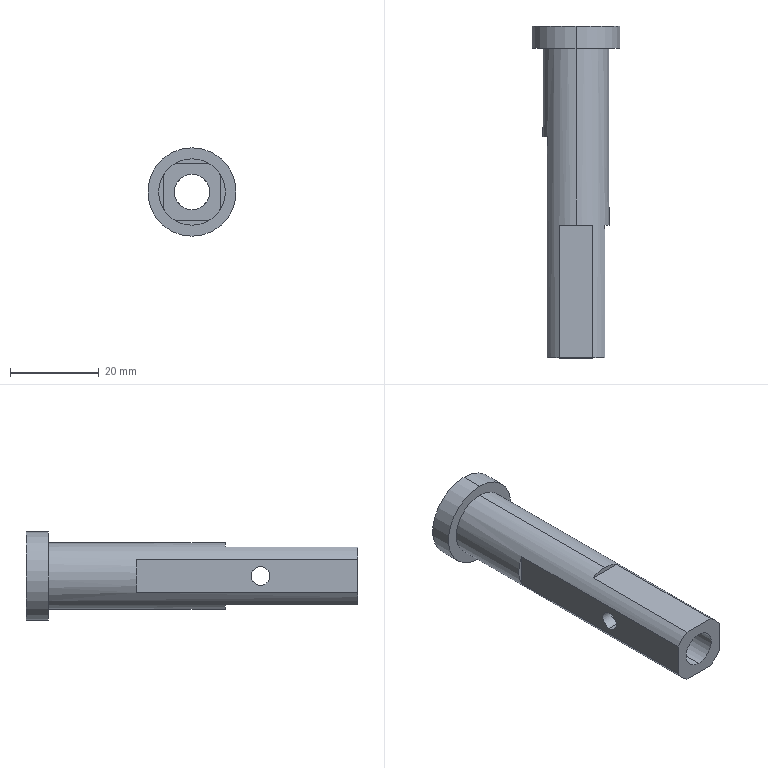Part | SolidWorks | features BaseBody 1 | 1 solid | 21 faces | box 20 x 75 x 20 mm | volume 9389 mm3 | plane 11 | cylinder 10 | commonest cylinder face diameters 4.2 x4 8 x2 15 x2 20 x2
STEP:
#1=CARTESIAN_POINT('',(-6.5,22.,2.1));
#2=VERTEX_POINT('',#1);
#3=CARTESIAN_POINT('',(-3.404,22.,2.1));
#4=VERTEX_POINT('',#3);
#5=CARTESIAN_POINT('',(6.5,22.,2.1));
#6=DIRECTION('',(1.,0.,0.));
#7=VECTOR('',#6,1000.);
#8=LINE('',#5,#7);
#9=EDGE_CURVE('',#2,#4,#8,.T.);
#10=ORIENTED_EDGE('',*,*,#9,.F.);
#11=CARTESIAN_POINT('',(-6.5,22.,-2.1));
#12=VERTEX_POINT('',#11);
#13=CARTESIAN_POINT('',(-6.5,22.,0.));
#14=DIRECTION('',(1.,0.,0.));
#15=DIRECTION('',(0.,0.,-1.));
#16=AXIS2_PLACEMENT_3D('',#13,#14,#15);
#17=CIRCLE('',#16,2.1);
#18=EDGE_CURVE('',#12,#2,#17,.T.);
#19=ORIENTED_EDGE('',*,*,#18,.F.);
#20=CARTESIAN_POINT('',(-3.404,22.,-2.1));
#21=VERTEX_POINT('',#20);
#22=CARTESIAN_POINT('',(6.5,22.,-2.1));
#23=DIRECTION('',(1.,0.,0.));
#24=VECTOR('',#23,1000.);
#25=LINE('',#22,#24);
#26=EDGE_CURVE('',#12,#21,#25,.T.);
#27=ORIENTED_EDGE('',*,*,#26,.T.);
#28=CARTESIAN_POINT('',(-3.404,22.,2.1));
#29=CARTESIAN_POINT('',(-3.404,22.139,2.1));
#30=CARTESIAN_POINT('',(-3.413,22.277,2.087));
#31=CARTESIAN_POINT('',(-3.437,22.48,2.046));
#32=CARTESIAN_POINT('',(-3.447,22.547,2.029));
#33=CARTESIAN_POINT('',(-3.465,22.647,1.998));
#34=CARTESIAN_POINT('',(-3.472,22.681,1.987));
#35=CARTESIAN_POINT('',(-3.485,22.747,1.963));
#36=CARTESIAN_POINT('',(-3.493,22.782,1.949));
#37=CARTESIAN_POINT('',(-3.529,22.938,1.884));
#38=CARTESIAN_POINT('',(-3.563,23.056,1.821));
#39=CARTESIAN_POINT('',(-3.617,23.224,1.708));
#40=CARTESIAN_POINT('',(-3.636,23.278,1.668));
#41=CARTESIAN_POINT('',(-3.675,23.384,1.581));
#42=CARTESIAN_POINT('',(-3.695,23.436,1.534));
#43=CARTESIAN_POINT('',(-3.753,23.582,1.388));
#44=CARTESIAN_POINT('',(-3.79,23.668,1.284));
#45=CARTESIAN_POINT('',(-3.842,23.781,1.116));
#46=CARTESIAN_POINT('',(-3.858,23.816,1.058));
#47=CARTESIAN_POINT('',(-3.889,23.88,0.9387));
#48=CARTESIAN_POINT('',(-3.903,23.909,0.8786));
#49=CARTESIAN_POINT('',(-3.97,24.045,0.5543));
#50=CARTESIAN_POINT('',(-4.,24.1,0.2829));
#51=CARTESIAN_POINT('',(-4.,24.1,-0.138));
#52=CARTESIAN_POINT('',(-3.993,24.087,-0.2764));
#53=CARTESIAN_POINT('',(-3.972,24.046,-0.4803));
#54=CARTESIAN_POINT('',(-3.963,24.029,-0.5476));
#55=CARTESIAN_POINT('',(-3.942,23.988,-0.6808));
#56=CARTESIAN_POINT('',(-3.93,23.963,-0.7482));
#57=CARTESIAN_POINT('',(-3.89,23.883,-0.9392));
#58=CARTESIAN_POINT('',(-3.859,23.819,-1.059));
#59=CARTESIAN_POINT('',(-3.79,23.668,-1.284));
#60=CARTESIAN_POINT('',(-3.753,23.582,-1.388));
#61=CARTESIAN_POINT('',(-3.674,23.385,-1.585));
#62=CARTESIAN_POINT('',(-3.635,23.279,-1.671));
#63=CARTESIAN_POINT('',(-3.581,23.112,-1.783));
#64=CARTESIAN_POINT('',(-3.563,23.054,-1.818));
#65=CARTESIAN_POINT('',(-3.538,22.966,-1.865));
#66=CARTESIAN_POINT('',(-3.53,22.936,-1.881));
#67=CARTESIAN_POINT('',(-3.515,22.875,-1.909));
#68=CARTESIAN_POINT('',(-3.508,22.846,-1.922));
#69=CARTESIAN_POINT('',(-3.439,22.55,-2.047));
#70=CARTESIAN_POINT('',(-3.404,22.279,-2.1));
#71=CARTESIAN_POINT('',(-3.404,22.,-2.1));
#72=B_SPLINE_CURVE_WITH_KNOTS('',3,(#28,#29,#30,#31,#32,#33,#34,#35,#36,#37,#38,#39,#40,#41,#42,#43,#44,#45,#46,#47,#48,#49,#50,#51,#52,#53,#54,#55,#56,#57,#58,#59,#60,#61,#62,#63,#64,#65,#66,#67,#68,#69,#70,#71),.UNSPECIFIED.,.F.,.F.,(4,2,2,2,2,2,2,2,2,2,2,2,2,2,2,2,2,2,2,2,2,4),(0.,0.0625,0.09375,0.1094,0.125,0.1875,0.2188,0.25,0.3125,0.3438,0.375,0.5,0.5625,0.5938,0.625,0.6875,0.75,0.8125,0.8438,0.8594,0.875,1.),.UNSPECIFIED.);
#73=EDGE_CURVE('',#4,#21,#72,.T.);
#74=ORIENTED_EDGE('',*,*,#73,.F.);
#75=EDGE_LOOP('',(#10,#19,#27,#74));
#76=FACE_OUTER_BOUND('',#75,.T.);
#77=CARTESIAN_POINT('',(6.5,22.,0.));
#78=DIRECTION('',(1.,0.,0.));
#79=DIRECTION('',(0.,0.,-1.));
#80=AXIS2_PLACEMENT_3D('',#77,#78,#79);
#81=CYLINDRICAL_SURFACE('',#80,2.1);
#82=ADVANCED_FACE('',(#76),#81,.F.);
#83=CARTESIAN_POINT('',(3.404,22.,2.1));
#84=VERTEX_POINT('',#83);
#85=CARTESIAN_POINT('',(6.5,22.,2.1));
#86=VERTEX_POINT('',#85);
#87=CARTESIAN_POINT('',(6.5,22.,2.1));
#88=DIRECTION('',(1.,0.,0.));
#89=VECTOR('',#88,1000.);
#90=LINE('',#87,#89);
#91=EDGE_CURVE('',#84,#86,#90,.T.);
#92=ORIENTED_EDGE('',*,*,#91,.F.);
#93=CARTESIAN_POINT('',(3.404,22.,-2.1));
#94=VERTEX_POINT('',#93);
#95=CARTESIAN_POINT('',(3.404,22.,-2.1));
#96=CARTESIAN_POINT('',(3.404,22.139,-2.1));
#97=CARTESIAN_POINT('',(3.413,22.277,-2.087));
#98=CARTESIAN_POINT('',(3.437,22.48,-2.046));
#99=CARTESIAN_POINT('',(3.447,22.547,-2.029));
#100=CARTESIAN_POINT('',(3.465,22.647,-1.998));
#101=CARTESIAN_POINT('',(3.472,22.681,-1.987));
#102=CARTESIAN_POINT('',(3.485,22.747,-1.963));
#103=CARTESIAN_POINT('',(3.493,22.782,-1.949));
#104=CARTESIAN_POINT('',(3.515,22.875,-1.91));
#105=CARTESIAN_POINT('',(3.53,22.936,-1.881));
#106=CARTESIAN_POINT('',(3.564,23.056,-1.817));
#107=CARTESIAN_POINT('',(3.582,23.116,-1.78));
#108=CARTESIAN_POINT('',(3.637,23.284,-1.667));
#109=CARTESIAN_POINT('',(3.675,23.388,-1.582));
#110=CARTESIAN_POINT('',(3.752,23.58,-1.39));
#111=CARTESIAN_POINT('',(3.79,23.666,-1.286));
#112=CARTESIAN_POINT('',(3.842,23.78,-1.116));
#113=CARTESIAN_POINT('',(3.858,23.815,-1.058));
#114=CARTESIAN_POINT('',(3.881,23.864,-0.968));
#115=CARTESIAN_POINT('',(3.889,23.879,-0.9378));
#116=CARTESIAN_POINT('',(3.903,23.909,-0.8765));
#117=CARTESIAN_POINT('',(3.91,23.922,-0.8465));
#118=CARTESIAN_POINT('',(3.97,24.045,-0.5542));
#119=CARTESIAN_POINT('',(4.,24.1,-0.2827));
#120=CARTESIAN_POINT('',(4.,24.1,0.1391));
#121=CARTESIAN_POINT('',(3.993,24.086,0.2779));
#122=CARTESIAN_POINT('',(3.971,24.045,0.4822));
#123=CARTESIAN_POINT('',(3.958,24.02,0.5833));
#124=CARTESIAN_POINT('',(3.941,23.986,0.6829));
#125=CARTESIAN_POINT('',(3.929,23.962,0.7489));
#126=CARTESIAN_POINT('',(3.923,23.949,0.7827));
#127=CARTESIAN_POINT('',(3.864,23.83,1.067));
#128=CARTESIAN_POINT('',(3.79,23.675,1.296));
#129=CARTESIAN_POINT('',(3.694,23.434,1.536));
#130=CARTESIAN_POINT('',(3.675,23.384,1.581));
#131=CARTESIAN_POINT('',(3.637,23.28,1.666));
#132=CARTESIAN_POINT('',(3.618,23.227,1.706));
#133=CARTESIAN_POINT('',(3.581,23.112,1.783));
#134=CARTESIAN_POINT('',(3.563,23.053,1.818));
#135=CARTESIAN_POINT('',(3.538,22.964,1.866));
#136=CARTESIAN_POINT('',(3.53,22.934,1.881));
#137=CARTESIAN_POINT('',(3.514,22.873,1.91));
#138=CARTESIAN_POINT('',(3.507,22.844,1.923));
#139=CARTESIAN_POINT('',(3.439,22.548,2.047));
#140=CARTESIAN_POINT('',(3.404,22.278,2.1));
#141=CARTESIAN_POINT('',(3.404,22.,2.1));
#142=B_SPLINE_CURVE_WITH_KNOTS('',3,(#95,#96,#97,#98,#99,#100,#101,#102,#103,#104,#105,#106,#107,#108,#109,#110,#111,#112,#113,#114,#115,#116,#117,#118,#119,#120,#121,#122,#123,#124,#125,#126,#127,#128,#129,#130,#131,#132,#133,#134,#135,#136,#137,#138,#139,#140,#141),.UNSPECIFIED.,.F.,.F.,(4,2,2,2,2,2,2,2,2,2,2,2,2,2,1,2,2,2,2,2,2,2,2,4),(0.,0.0625,0.09375,0.1094,0.125,0.1562,0.1875,0.25,0.3125,0.3437,0.3594,0.375,0.5,0.5625,0.5937,0.6094,0.625,0.75,0.7813,0.8125,0.8438,0.8594,0.875,1.),.UNSPECIFIED.);
#143=EDGE_CURVE('',#94,#84,#142,.T.);
#144=ORIENTED_EDGE('',*,*,#143,.F.);
#145=CARTESIAN_POINT('',(6.5,22.,-2.1));
#146=VERTEX_POINT('',#145);
#147=CARTESIAN_POINT('',(6.5,22.,-2.1));
#148=DIRECTION('',(1.,0.,0.));
#149=VECTOR('',#148,1000.);
#150=LINE('',#147,#149);
#151=EDGE_CURVE('',#94,#146,#150,.T.);
#152=ORIENTED_EDGE('',*,*,#151,.T.);
#153=CARTESIAN_POINT('',(6.5,22.,0.));
#154=DIRECTION('',(1.,0.,0.));
#155=DIRECTION('',(0.,0.,-1.));
#156=AXIS2_PLACEMENT_3D('',#153,#154,#155);
#157=CIRCLE('',#156,2.1);
#158=EDGE_CURVE('',#146,#86,#157,.T.);
#159=ORIENTED_EDGE('',*,*,#158,.T.);
#160=EDGE_LOOP('',(#92,#144,#152,#159));
#161=FACE_OUTER_BOUND('',#160,.T.);
#162=CARTESIAN_POINT('',(6.5,22.,0.));
#163=DIRECTION('',(1.,0.,0.));
#164=DIRECTION('',(0.,0.,-1.));
#165=AXIS2_PLACEMENT_3D('',#162,#163,#164);
#166=CYLINDRICAL_SURFACE('',#165,2.1);
#167=ADVANCED_FACE('',(#161),#166,.F.);
#168=CARTESIAN_POINT('',(-3.742,30.,6.5));
#169=VERTEX_POINT('',#168);
#170=CARTESIAN_POINT('',(3.742,30.,6.5));
#171=VERTEX_POINT('',#170);
#172=CARTESIAN_POINT('',(-5.,30.,6.5));
#173=DIRECTION('',(1.,0.,0.));
#174=VECTOR('',#173,1000.);
#175=LINE('',#172,#174);
#176=EDGE_CURVE('',#169,#171,#175,.T.);
#177=ORIENTED_EDGE('',*,*,#176,.T.);
#178=CARTESIAN_POINT('',(0.,30.,7.5));
#179=VERTEX_POINT('',#178);
#180=CARTESIAN_POINT('',(0.,30.,0.));
#181=DIRECTION('',(0.,1.,0.));
#182=DIRECTION('',(0.,0.,1.));
#183=AXIS2_PLACEMENT_3D('',#180,#181,#182);
#184=CIRCLE('',#183,7.5);
#185=EDGE_CURVE('',#179,#171,#184,.T.);
#186=ORIENTED_EDGE('',*,*,#185,.F.);
#187=CARTESIAN_POINT('',(0.,30.,0.));
#188=DIRECTION('',(0.,1.,0.));
#189=DIRECTION('',(0.,0.,1.));
#190=AXIS2_PLACEMENT_3D('',#187,#188,#189);
#191=CIRCLE('',#190,7.5);
#192=EDGE_CURVE('',#169,#179,#191,.T.);
#193=ORIENTED_EDGE('',*,*,#192,.F.);
#194=EDGE_LOOP('',(#177,#186,#193));
#195=FACE_OUTER_BOUND('',#194,.T.);
#196=CARTESIAN_POINT('',(0.,30.,0.));
#197=DIRECTION('',(0.,1.,0.));
#198=DIRECTION('',(1.,0.,0.));
#199=AXIS2_PLACEMENT_3D('',#196,#197,#198);
#200=PLANE('',#199);
#201=ADVANCED_FACE('',(#195),#200,.F.);
#202=ORIENTED_EDGE('',*,*,#176,.F.);
#203=CARTESIAN_POINT('',(-3.742,0.,6.5));
#204=VERTEX_POINT('',#203);
#205=CARTESIAN_POINT('',(-3.742,0.,6.5));
#206=DIRECTION('',(0.,1.,0.));
#207=VECTOR('',#206,1000.);
#208=LINE('',#205,#207);
#209=EDGE_CURVE('',#204,#169,#208,.T.);
#210=ORIENTED_EDGE('',*,*,#209,.F.);
#211=CARTESIAN_POINT('',(3.742,0.,6.5));
#212=VERTEX_POINT('',#211);
#213=CARTESIAN_POINT('',(-5.,0.,6.5));
#214=DIRECTION('',(1.,0.,0.));
#215=VECTOR('',#214,1000.);
#216=LINE('',#213,#215);
#217=EDGE_CURVE('',#204,#212,#216,.T.);
#218=ORIENTED_EDGE('',*,*,#217,.T.);
#219=CARTESIAN_POINT('',(3.742,0.,6.5));
#220=DIRECTION('',(0.,-1.,0.));
#221=VECTOR('',#220,1000.);
#222=LINE('',#219,#221);
#223=EDGE_CURVE('',#171,#212,#222,.T.);
#224=ORIENTED_EDGE('',*,*,#223,.F.);
#225=EDGE_LOOP('',(#202,#210,#218,#224));
#226=FACE_OUTER_BOUND('',#225,.T.);
#227=CARTESIAN_POINT('',(-5.,30.,6.5));
#228=DIRECTION('',(0.,0.,-1.));
#229=DIRECTION('',(0.,-1.,0.));
#230=AXIS2_PLACEMENT_3D('',#227,#228,#229);
#231=PLANE('',#230);
#232=ADVANCED_FACE('',(#226),#231,.F.);
#233=CARTESIAN_POINT('',(-3.742,30.,-6.5));
#234=VERTEX_POINT('',#233);
#235=CARTESIAN_POINT('',(0.,30.,-7.5));
#236=VERTEX_POINT('',#235);
#237=CARTESIAN_POINT('',(0.,30.,0.));
#238=DIRECTION('',(0.,-1.,0.));
#239=DIRECTION('',(0.,0.,-1.));
#240=AXIS2_PLACEMENT_3D('',#237,#238,#239);
#241=CIRCLE('',#240,7.5);
#242=EDGE_CURVE('',#234,#236,#241,.T.);
#243=ORIENTED_EDGE('',*,*,#242,.T.);
#244=CARTESIAN_POINT('',(3.742,30.,-6.5));
#245=VERTEX_POINT('',#244);
#246=CARTESIAN_POINT('',(0.,30.,0.));
#247=DIRECTION('',(0.,-1.,0.));
#248=DIRECTION('',(0.,0.,-1.));
#249=AXIS2_PLACEMENT_3D('',#246,#247,#248);
#250=CIRCLE('',#249,7.5);
#251=EDGE_CURVE('',#236,#245,#250,.T.);
#252=ORIENTED_EDGE('',*,*,#251,.T.);
#253=CARTESIAN_POINT('',(-5.,30.,-6.5));
#254=DIRECTION('',(-1.,0.,0.));
#255=VECTOR('',#254,1000.);
#256=LINE('',#253,#255);
#257=EDGE_CURVE('',#245,#234,#256,.T.);
#258=ORIENTED_EDGE('',*,*,#257,.T.);
#259=EDGE_LOOP('',(#243,#252,#258));
#260=FACE_OUTER_BOUND('',#259,.T.);
#261=CARTESIAN_POINT('',(0.,30.,0.));
#262=DIRECTION('',(0.,-1.,0.));
#263=DIRECTION('',(0.,0.,-1.));
#264=AXIS2_PLACEMENT_3D('',#261,#262,#263);
#265=PLANE('',#264);
#266=ADVANCED_FACE('',(#260),#265,.T.);
#267=ORIENTED_EDGE('',*,*,#257,.F.);
#268=CARTESIAN_POINT('',(3.742,0.,-6.5));
#269=VERTEX_POINT('',#268);
#270=CARTESIAN_POINT('',(3.742,0.,-6.5));
#271=DIRECTION('',(0.,1.,0.));
#272=VECTOR('',#271,1000.);
#273=LINE('',#270,#272);
#274=EDGE_CURVE('',#269,#245,#273,.T.);
#275=ORIENTED_EDGE('',*,*,#274,.F.);
#276=CARTESIAN_POINT('',(-3.742,0.,-6.5));
#277=VERTEX_POINT('',#276);
#278=CARTESIAN_POINT('',(-5.,0.,-6.5));
#279=DIRECTION('',(-1.,0.,0.));
#280=VECTOR('',#279,1000.);
#281=LINE('',#278,#280);
#282=EDGE_CURVE('',#269,#277,#281,.T.);
#283=ORIENTED_EDGE('',*,*,#282,.T.);
#284=CARTESIAN_POINT('',(-3.742,0.,-6.5));
#285=DIRECTION('',(0.,-1.,0.));
#286=VECTOR('',#285,1000.);
#287=LINE('',#284,#286);
#288=EDGE_CURVE('',#234,#277,#287,.T.);
#289=ORIENTED_EDGE('',*,*,#288,.F.);
#290=EDGE_LOOP('',(#267,#275,#283,#289));
#291=FACE_OUTER_BOUND('',#290,.T.);
#292=CARTESIAN_POINT('',(-5.,30.,-6.5));
#293=DIRECTION('',(0.,0.,1.));
#294=DIRECTION('',(1.,0.,0.));
#295=AXIS2_PLACEMENT_3D('',#292,#293,#294);
#296=PLANE('',#295);
#297=ADVANCED_FACE('',(#291),#296,.F.);
#298=CARTESIAN_POINT('',(6.5,30.,3.742));
#299=VERTEX_POINT('',#298);
#300=CARTESIAN_POINT('',(6.5,30.,-3.742));
#301=VERTEX_POINT('',#300);
#302=CARTESIAN_POINT('',(6.5,30.,-5.));
#303=DIRECTION('',(0.,0.,-1.));
#304=VECTOR('',#303,1000.);
#305=LINE('',#302,#304);
#306=EDGE_CURVE('',#299,#301,#305,.T.);
#307=ORIENTED_EDGE('',*,*,#306,.T.);
#308=CARTESIAN_POINT('',(0.,30.,0.));
#309=DIRECTION('',(0.,1.,0.));
#310=DIRECTION('',(0.,0.,1.));
#311=AXIS2_PLACEMENT_3D('',#308,#309,#310);
#312=CIRCLE('',#311,7.5);
#313=EDGE_CURVE('',#299,#301,#312,.T.);
#314=ORIENTED_EDGE('',*,*,#313,.F.);
#315=EDGE_LOOP('',(#307,#314));
#316=FACE_OUTER_BOUND('',#315,.T.);
#317=CARTESIAN_POINT('',(0.,30.,0.));
#318=DIRECTION('',(0.,1.,0.));
#319=DIRECTION('',(1.,0.,0.));
#320=AXIS2_PLACEMENT_3D('',#317,#318,#319);
#321=PLANE('',#320);
#322=ADVANCED_FACE('',(#316),#321,.F.);
#323=ORIENTED_EDGE('',*,*,#158,.F.);
#324=CARTESIAN_POINT('',(6.5,22.,0.));
#325=DIRECTION('',(1.,0.,0.));
#326=DIRECTION('',(0.,0.,-1.));
#327=AXIS2_PLACEMENT_3D('',#324,#325,#326);
#328=CIRCLE('',#327,2.1);
#329=EDGE_CURVE('',#86,#146,#328,.T.);
#330=ORIENTED_EDGE('',*,*,#329,.F.);
#331=EDGE_LOOP('',(#323,#330));
#332=FACE_BOUND('',#331,.T.);
#333=ORIENTED_EDGE('',*,*,#306,.F.);
#334=CARTESIAN_POINT('',(6.5,0.,3.742));
#335=VERTEX_POINT('',#334);
#336=CARTESIAN_POINT('',(6.5,0.,3.742));
#337=DIRECTION('',(0.,1.,0.));
#338=VECTOR('',#337,1000.);
#339=LINE('',#336,#338);
#340=EDGE_CURVE('',#335,#299,#339,.T.);
#341=ORIENTED_EDGE('',*,*,#340,.F.);
#342=CARTESIAN_POINT('',(6.5,0.,-3.742));
#343=VERTEX_POINT('',#342);
#344=CARTESIAN_POINT('',(6.5,0.,-5.));
#345=DIRECTION('',(0.,0.,-1.));
#346=VECTOR('',#345,1000.);
#347=LINE('',#344,#346);
#348=EDGE_CURVE('',#335,#343,#347,.T.);
#349=ORIENTED_EDGE('',*,*,#348,.T.);
#350=CARTESIAN_POINT('',(6.5,0.,-3.742));
#351=DIRECTION('',(0.,-1.,0.));
#352=VECTOR('',#351,1000.);
#353=LINE('',#350,#352);
#354=EDGE_CURVE('',#301,#343,#353,.T.);
#355=ORIENTED_EDGE('',*,*,#354,.F.);
#356=EDGE_LOOP('',(#333,#341,#349,#355));
#357=FACE_OUTER_BOUND('',#356,.T.);
#358=CARTESIAN_POINT('',(6.5,30.,-5.));
#359=DIRECTION('',(-1.,0.,0.));
#360=DIRECTION('',(0.,0.,1.));
#361=AXIS2_PLACEMENT_3D('',#358,#359,#360);
#362=PLANE('',#361);
#363=ADVANCED_FACE('',(#332,#357),#362,.F.);
#364=CARTESIAN_POINT('',(-6.5,50.,3.742));
#365=VERTEX_POINT('',#364);
#366=CARTESIAN_POINT('',(-6.5,50.,-3.742));
#367=VERTEX_POINT('',#366);
#368=CARTESIAN_POINT('',(0.,50.,0.));
#369=DIRECTION('',(0.,-1.,0.));
#370=DIRECTION('',(0.,0.,-1.));
#371=AXIS2_PLACEMENT_3D('',#368,#369,#370);
#372=CIRCLE('',#371,7.5);
#373=EDGE_CURVE('',#365,#367,#372,.T.);
#374=ORIENTED_EDGE('',*,*,#373,.T.);
#375=CARTESIAN_POINT('',(-6.5,50.,0.));
#376=DIRECTION('',(0.,0.,1.));
#377=VECTOR('',#376,1000.);
#378=LINE('',#375,#377);
#379=EDGE_CURVE('',#367,#365,#378,.T.);
#380=ORIENTED_EDGE('',*,*,#379,.T.);
#381=EDGE_LOOP('',(#374,#380));
#382=FACE_OUTER_BOUND('',#381,.T.);
#383=CARTESIAN_POINT('',(0.,50.,0.));
#384=DIRECTION('',(0.,-1.,0.));
#385=DIRECTION('',(0.,0.,-1.));
#386=AXIS2_PLACEMENT_3D('',#383,#384,#385);
#387=PLANE('',#386);
#388=ADVANCED_FACE('',(#382),#387,.T.);
#389=ORIENTED_EDGE('',*,*,#18,.T.);
#390=CARTESIAN_POINT('',(-6.5,22.,0.));
#391=DIRECTION('',(1.,0.,0.));
#392=DIRECTION('',(0.,0.,-1.));
#393=AXIS2_PLACEMENT_3D('',#390,#391,#392);
#394=CIRCLE('',#393,2.1);
#395=EDGE_CURVE('',#2,#12,#394,.T.);
#396=ORIENTED_EDGE('',*,*,#395,.T.);
#397=EDGE_LOOP('',(#389,#396));
#398=FACE_BOUND('',#397,.T.);
#399=ORIENTED_EDGE('',*,*,#379,.F.);
#400=CARTESIAN_POINT('',(-6.5,0.,-3.742));
#401=VERTEX_POINT('',#400);
#402=CARTESIAN_POINT('',(-6.5,0.,-3.742));
#403=DIRECTION('',(0.,1.,0.));
#404=VECTOR('',#403,1000.);
#405=LINE('',#402,#404);
#406=EDGE_CURVE('',#401,#367,#405,.T.);
#407=ORIENTED_EDGE('',*,*,#406,.F.);
#408=CARTESIAN_POINT('',(-6.5,0.,3.742));
#409=VERTEX_POINT('',#408);
#410=CARTESIAN_POINT('',(-6.5,0.,-5.));
#411=DIRECTION('',(0.,0.,1.));
#412=VECTOR('',#411,1000.);
#413=LINE('',#410,#412);
#414=EDGE_CURVE('',#401,#409,#413,.T.);
#415=ORIENTED_EDGE('',*,*,#414,.T.);
#416=CARTESIAN_POINT('',(-6.5,0.,3.742));
#417=DIRECTION('',(0.,-1.,0.));
#418=VECTOR('',#417,1000.);
#419=LINE('',#416,#418);
#420=EDGE_CURVE('',#365,#409,#419,.T.);
#421=ORIENTED_EDGE('',*,*,#420,.F.);
#422=EDGE_LOOP('',(#399,#407,#415,#421));
#423=FACE_OUTER_BOUND('',#422,.T.);
#424=CARTESIAN_POINT('',(-6.5,30.,-5.));
#425=DIRECTION('',(1.,0.,0.));
#426=DIRECTION('',(0.,1.,0.));
#427=AXIS2_PLACEMENT_3D('',#424,#425,#426);
#428=PLANE('',#427);
#429=ADVANCED_FACE('',(#398,#423),#428,.F.);
#430=ORIENTED_EDGE('',*,*,#143,.T.);
#431=CARTESIAN_POINT('',(3.404,22.,2.1));
#432=CARTESIAN_POINT('',(3.404,21.861,2.1));
#433=CARTESIAN_POINT('',(3.413,21.723,2.087));
#434=CARTESIAN_POINT('',(3.437,21.52,2.046));
#435=CARTESIAN_POINT('',(3.447,21.453,2.029));
#436=CARTESIAN_POINT('',(3.465,21.353,1.998));
#437=CARTESIAN_POINT('',(3.472,21.319,1.987));
#438=CARTESIAN_POINT('',(3.485,21.253,1.963));
#439=CARTESIAN_POINT('',(3.493,21.218,1.949));
#440=CARTESIAN_POINT('',(3.529,21.062,1.884));
#441=CARTESIAN_POINT('',(3.563,20.944,1.821));
#442=CARTESIAN_POINT('',(3.617,20.776,1.708));
#443=CARTESIAN_POINT('',(3.636,20.722,1.668));
#444=CARTESIAN_POINT('',(3.675,20.616,1.581));
#445=CARTESIAN_POINT('',(3.695,20.564,1.534));
#446=CARTESIAN_POINT('',(3.753,20.418,1.388));
#447=CARTESIAN_POINT('',(3.79,20.332,1.284));
#448=CARTESIAN_POINT('',(3.842,20.219,1.116));
#449=CARTESIAN_POINT('',(3.858,20.184,1.058));
#450=CARTESIAN_POINT('',(3.889,20.12,0.9387));
#451=CARTESIAN_POINT('',(3.903,20.091,0.8786));
#452=CARTESIAN_POINT('',(3.97,19.955,0.5543));
#453=CARTESIAN_POINT('',(4.,19.9,0.2829));
#454=CARTESIAN_POINT('',(4.,19.9,-0.138));
#455=CARTESIAN_POINT('',(3.993,19.913,-0.2764));
#456=CARTESIAN_POINT('',(3.972,19.954,-0.4803));
#457=CARTESIAN_POINT('',(3.963,19.971,-0.5476));
#458=CARTESIAN_POINT('',(3.942,20.012,-0.6808));
#459=CARTESIAN_POINT('',(3.93,20.037,-0.7482));
#460=CARTESIAN_POINT('',(3.89,20.117,-0.9392));
#461=CARTESIAN_POINT('',(3.859,20.181,-1.059));
#462=CARTESIAN_POINT('',(3.79,20.332,-1.284));
#463=CARTESIAN_POINT('',(3.753,20.418,-1.388));
#464=CARTESIAN_POINT('',(3.674,20.615,-1.585));
#465=CARTESIAN_POINT('',(3.635,20.721,-1.671));
#466=CARTESIAN_POINT('',(3.581,20.888,-1.783));
#467=CARTESIAN_POINT('',(3.563,20.946,-1.818));
#468=CARTESIAN_POINT('',(3.538,21.034,-1.865));
#469=CARTESIAN_POINT('',(3.53,21.064,-1.881));
#470=CARTESIAN_POINT('',(3.515,21.125,-1.909));
#471=CARTESIAN_POINT('',(3.508,21.154,-1.922));
#472=CARTESIAN_POINT('',(3.439,21.45,-2.047));
#473=CARTESIAN_POINT('',(3.404,21.721,-2.1));
#474=CARTESIAN_POINT('',(3.404,22.,-2.1));
#475=B_SPLINE_CURVE_WITH_KNOTS('',3,(#431,#432,#433,#434,#435,#436,#437,#438,#439,#440,#441,#442,#443,#444,#445,#446,#447,#448,#449,#450,#451,#452,#453,#454,#455,#456,#457,#458,#459,#460,#461,#462,#463,#464,#465,#466,#467,#468,#469,#470,#471,#472,#473,#474),.UNSPECIFIED.,.F.,.F.,(4,2,2,2,2,2,2,2,2,2,2,2,2,2,2,2,2,2,2,2,2,4),(0.,0.0625,0.09375,0.1094,0.125,0.1875,0.2187,0.25,0.3125,0.3437,0.375,0.5,0.5625,0.5937,0.625,0.6875,0.75,0.8125,0.8437,0.8594,0.875,1.),.UNSPECIFIED.);
#476=EDGE_CURVE('',#84,#94,#475,.T.);
#477=ORIENTED_EDGE('',*,*,#476,.T.);
#478=EDGE_LOOP('',(#430,#477));
#479=FACE_BOUND('',#478,.T.);
#480=CARTESIAN_POINT('',(0.,0.,-4.));
#481=VERTEX_POINT('',#480);
#482=CARTESIAN_POINT('',(0.,75.,-4.));
#483=VERTEX_POINT('',#482);
#484=CARTESIAN_POINT('',(0.,-11.314,-4.));
#485=DIRECTION('',(0.,1.,0.));
#486=VECTOR('',#485,1000.);
#487=LINE('',#484,#486);
#488=EDGE_CURVE('',#481,#483,#487,.T.);
#489=ORIENTED_EDGE('',*,*,#488,.F.);
#490=CARTESIAN_POINT('',(0.,0.,4.));
#491=VERTEX_POINT('',#490);
#492=CARTESIAN_POINT('',(0.,0.,0.));
#493=DIRECTION('',(0.,-1.,0.));
#494=DIRECTION('',(0.,0.,1.));
#495=AXIS2_PLACEMENT_3D('',#492,#493,#494);
#496=CIRCLE('',#495,4.);
#497=EDGE_CURVE('',#481,#491,#496,.T.);
#498=ORIENTED_EDGE('',*,*,#497,.T.);
#499=CARTESIAN_POINT('',(0.,75.,4.));
#500=VERTEX_POINT('',#499);
#501=CARTESIAN_POINT('',(0.,-11.314,4.));
#502=DIRECTION('',(0.,1.,0.));
#503=VECTOR('',#502,1000.);
#504=LINE('',#501,#503);
#505=EDGE_CURVE('',#491,#500,#504,.T.);
#506=ORIENTED_EDGE('',*,*,#505,.T.);
#507=CARTESIAN_POINT('',(0.,75.,0.));
#508=DIRECTION('',(0.,1.,0.));
#509=DIRECTION('',(0.,0.,1.));
#510=AXIS2_PLACEMENT_3D('',#507,#508,#509);
#511=CIRCLE('',#510,4.);
#512=EDGE_CURVE('',#500,#483,#511,.T.);
#513=ORIENTED_EDGE('',*,*,#512,.T.);
#514=EDGE_LOOP('',(#489,#498,#506,#513));
#515=FACE_OUTER_BOUND('',#514,.T.);
#516=CARTESIAN_POINT('',(0.,-11.314,0.));
#517=DIRECTION('',(0.,1.,0.));
#518=DIRECTION('',(0.,0.,1.));
#519=AXIS2_PLACEMENT_3D('',#516,#517,#518);
#520=CYLINDRICAL_SURFACE('',#519,4.);
#521=ADVANCED_FACE('',(#479,#515),#520,.F.);
#522=CARTESIAN_POINT('',(0.,70.,7.5));
#523=VERTEX_POINT('',#522);
#524=CARTESIAN_POINT('',(0.,0.,7.5));
#525=DIRECTION('',(0.,-1.,0.));
#526=VECTOR('',#525,1000.);
#527=LINE('',#524,#526);
#528=EDGE_CURVE('',#523,#179,#527,.T.);
#529=ORIENTED_EDGE('',*,*,#528,.F.);
#530=CARTESIAN_POINT('',(0.,70.,-7.5));
#531=VERTEX_POINT('',#530);
#532=CARTESIAN_POINT('',(0.,70.,0.));
#533=DIRECTION('',(0.,-1.,0.));
#534=DIRECTION('',(0.,0.,-1.));
#535=AXIS2_PLACEMENT_3D('',#532,#533,#534);
#536=CIRCLE('',#535,7.5);
#537=EDGE_CURVE('',#523,#531,#536,.T.);
#538=ORIENTED_EDGE('',*,*,#537,.T.);
#539=CARTESIAN_POINT('',(0.,0.,-7.5));
#540=DIRECTION('',(0.,-1.,0.));
#541=VECTOR('',#540,1000.);
#542=LINE('',#539,#541);
#543=EDGE_CURVE('',#531,#236,#542,.T.);
#544=ORIENTED_EDGE('',*,*,#543,.T.);
#545=ORIENTED_EDGE('',*,*,#242,.F.);
#546=ORIENTED_EDGE('',*,*,#288,.T.);
#547=CARTESIAN_POINT('',(0.,0.,0.));
#548=DIRECTION('',(0.,-1.,0.));
#549=DIRECTION('',(0.,0.,-1.));
#550=AXIS2_PLACEMENT_3D('',#547,#548,#549);
#551=CIRCLE('',#550,7.5);
#552=EDGE_CURVE('',#401,#277,#551,.T.);
#553=ORIENTED_EDGE('',*,*,#552,.F.);
#554=ORIENTED_EDGE('',*,*,#406,.T.);
#555=ORIENTED_EDGE('',*,*,#373,.F.);
#556=ORIENTED_EDGE('',*,*,#420,.T.);
#557=CARTESIAN_POINT('',(0.,0.,0.));
#558=DIRECTION('',(0.,-1.,0.));
#559=DIRECTION('',(0.,0.,-1.));
#560=AXIS2_PLACEMENT_3D('',#557,#558,#559);
#561=CIRCLE('',#560,7.5);
#562=EDGE_CURVE('',#204,#409,#561,.T.);
#563=ORIENTED_EDGE('',*,*,#562,.F.);
#564=ORIENTED_EDGE('',*,*,#209,.T.);
#565=ORIENTED_EDGE('',*,*,#192,.T.);
#566=EDGE_LOOP('',(#529,#538,#544,#545,#546,#553,#554,#555,#556,#563,#564,#565));
#567=FACE_OUTER_BOUND('',#566,.T.);
#568=CARTESIAN_POINT('',(0.,0.,0.));
#569=DIRECTION('',(0.,-1.,0.));
#570=DIRECTION('',(0.,0.,-1.));
#571=AXIS2_PLACEMENT_3D('',#568,#569,#570);
#572=CYLINDRICAL_SURFACE('',#571,7.5);
#573=ADVANCED_FACE('',(#567),#572,.T.);
#574=CARTESIAN_POINT('',(0.,70.,0.));
#575=DIRECTION('',(0.,-1.,0.));
#576=DIRECTION('',(0.,0.,-1.));
#577=AXIS2_PLACEMENT_3D('',#574,#575,#576);
#578=CIRCLE('',#577,7.5);
#579=EDGE_CURVE('',#531,#523,#578,.T.);
#580=ORIENTED_EDGE('',*,*,#579,.F.);
#581=ORIENTED_EDGE('',*,*,#537,.F.);
#582=EDGE_LOOP('',(#580,#581));
#583=FACE_BOUND('',#582,.T.);
#584=CARTESIAN_POINT('',(0.,70.,-10.));
#585=VERTEX_POINT('',#584);
#586=CARTESIAN_POINT('',(0.,70.,10.));
#587=VERTEX_POINT('',#586);
#588=CARTESIAN_POINT('',(0.,70.,0.));
#589=DIRECTION('',(0.,-1.,0.));
#590=DIRECTION('',(0.,0.,-1.));
#591=AXIS2_PLACEMENT_3D('',#588,#589,#590);
#592=CIRCLE('',#591,10.);
#593=EDGE_CURVE('',#585,#587,#592,.T.);
#594=ORIENTED_EDGE('',*,*,#593,.T.);
#595=CARTESIAN_POINT('',(0.,70.,0.));
#596=DIRECTION('',(0.,-1.,0.));
#597=DIRECTION('',(0.,0.,-1.));
#598=AXIS2_PLACEMENT_3D('',#595,#596,#597);
#599=CIRCLE('',#598,10.);
#600=EDGE_CURVE('',#587,#585,#599,.T.);
#601=ORIENTED_EDGE('',*,*,#600,.T.);
#602=EDGE_LOOP('',(#594,#601));
#603=FACE_OUTER_BOUND('',#602,.T.);
#604=CARTESIAN_POINT('',(-10.,70.,0.));
#605=DIRECTION('',(0.,1.,0.));
#606=DIRECTION('',(1.,0.,0.));
#607=AXIS2_PLACEMENT_3D('',#604,#605,#606);
#608=PLANE('',#607);
#609=ADVANCED_FACE('',(#583,#603),#608,.F.);
#610=CARTESIAN_POINT('',(0.,75.,10.));
#611=VERTEX_POINT('',#610);
#612=CARTESIAN_POINT('',(0.,0.,10.));
#613=DIRECTION('',(0.,-1.,0.));
#614=VECTOR('',#613,1000.);
#615=LINE('',#612,#614);
#616=EDGE_CURVE('',#611,#587,#615,.T.);
#617=ORIENTED_EDGE('',*,*,#616,.F.);
#618=CARTESIAN_POINT('',(0.,75.,-10.));
#619=VERTEX_POINT('',#618);
#620=CARTESIAN_POINT('',(0.,75.,0.));
#621=DIRECTION('',(0.,-1.,0.));
#622=DIRECTION('',(0.,0.,-1.));
#623=AXIS2_PLACEMENT_3D('',#620,#621,#622);
#624=CIRCLE('',#623,10.);
#625=EDGE_CURVE('',#611,#619,#624,.T.);
#626=ORIENTED_EDGE('',*,*,#625,.T.);
#627=CARTESIAN_POINT('',(0.,0.,-10.));
#628=DIRECTION('',(0.,-1.,0.));
#629=VECTOR('',#628,1000.);
#630=LINE('',#627,#629);
#631=EDGE_CURVE('',#619,#585,#630,.T.);
#632=ORIENTED_EDGE('',*,*,#631,.T.);
#633=ORIENTED_EDGE('',*,*,#600,.F.);
#634=EDGE_LOOP('',(#617,#626,#632,#633));
#635=FACE_OUTER_BOUND('',#634,.T.);
#636=CARTESIAN_POINT('',(0.,0.,0.));
#637=DIRECTION('',(0.,-1.,0.));
#638=DIRECTION('',(0.,0.,-1.));
#639=AXIS2_PLACEMENT_3D('',#636,#637,#638);
#640=CYLINDRICAL_SURFACE('',#639,10.);
#641=ADVANCED_FACE('',(#635),#640,.T.);
#642=ORIENTED_EDGE('',*,*,#512,.F.);
#643=CARTESIAN_POINT('',(0.,75.,0.));
#644=DIRECTION('',(0.,1.,0.));
#645=DIRECTION('',(0.,0.,1.));
#646=AXIS2_PLACEMENT_3D('',#643,#644,#645);
#647=CIRCLE('',#646,4.);
#648=EDGE_CURVE('',#483,#500,#647,.T.);
#649=ORIENTED_EDGE('',*,*,#648,.F.);
#650=EDGE_LOOP('',(#642,#649));
#651=FACE_BOUND('',#650,.T.);
#652=CARTESIAN_POINT('',(0.,75.,0.));
#653=DIRECTION('',(0.,-1.,0.));
#654=DIRECTION('',(0.,0.,-1.));
#655=AXIS2_PLACEMENT_3D('',#652,#653,#654);
#656=CIRCLE('',#655,10.);
#657=EDGE_CURVE('',#619,#611,#656,.T.);
#658=ORIENTED_EDGE('',*,*,#657,.F.);
#659=ORIENTED_EDGE('',*,*,#625,.F.);
#660=EDGE_LOOP('',(#658,#659));
#661=FACE_OUTER_BOUND('',#660,.T.);
#662=CARTESIAN_POINT('',(0.,75.,0.));
#663=DIRECTION('',(0.,-1.,0.));
#664=DIRECTION('',(0.,0.,-1.));
#665=AXIS2_PLACEMENT_3D('',#662,#663,#664);
#666=PLANE('',#665);
#667=ADVANCED_FACE('',(#651,#661),#666,.F.);
#668=CARTESIAN_POINT('',(0.,0.,0.));
#669=DIRECTION('',(0.,-1.,0.));
#670=DIRECTION('',(0.,0.,1.));
#671=AXIS2_PLACEMENT_3D('',#668,#669,#670);
#672=CIRCLE('',#671,4.);
#673=EDGE_CURVE('',#491,#481,#672,.T.);
#674=ORIENTED_EDGE('',*,*,#673,.F.);
#675=ORIENTED_EDGE('',*,*,#497,.F.);
#676=EDGE_LOOP('',(#674,#675));
#677=FACE_BOUND('',#676,.T.);
#678=CARTESIAN_POINT('',(0.,0.,0.));
#679=DIRECTION('',(0.,-1.,0.));
#680=DIRECTION('',(0.,0.,-1.));
#681=AXIS2_PLACEMENT_3D('',#678,#679,#680);
#682=CIRCLE('',#681,7.5);
#683=EDGE_CURVE('',#335,#212,#682,.T.);
#684=ORIENTED_EDGE('',*,*,#683,.T.);
#685=ORIENTED_EDGE('',*,*,#217,.F.);
#686=ORIENTED_EDGE('',*,*,#562,.T.);
#687=ORIENTED_EDGE('',*,*,#414,.F.);
#688=ORIENTED_EDGE('',*,*,#552,.T.);
#689=ORIENTED_EDGE('',*,*,#282,.F.);
#690=CARTESIAN_POINT('',(0.,0.,0.));
#691=DIRECTION('',(0.,-1.,0.));
#692=DIRECTION('',(0.,0.,-1.));
#693=AXIS2_PLACEMENT_3D('',#690,#691,#692);
#694=CIRCLE('',#693,7.5);
#695=EDGE_CURVE('',#269,#343,#694,.T.);
#696=ORIENTED_EDGE('',*,*,#695,.T.);
#697=ORIENTED_EDGE('',*,*,#348,.F.);
#698=EDGE_LOOP('',(#684,#685,#686,#687,#688,#689,#696,#697));
#699=FACE_OUTER_BOUND('',#698,.T.);
#700=CARTESIAN_POINT('',(-7.5,0.,0.));
#701=DIRECTION('',(0.,1.,0.));
#702=DIRECTION('',(1.,0.,0.));
#703=AXIS2_PLACEMENT_3D('',#700,#701,#702);
#704=PLANE('',#703);
#705=ADVANCED_FACE('',(#677,#699),#704,.F.);
#706=ORIENTED_EDGE('',*,*,#657,.T.);
#707=ORIENTED_EDGE('',*,*,#616,.T.);
#708=ORIENTED_EDGE('',*,*,#593,.F.);
#709=ORIENTED_EDGE('',*,*,#631,.F.);
#710=EDGE_LOOP('',(#706,#707,#708,#709));
#711=FACE_OUTER_BOUND('',#710,.T.);
#712=CARTESIAN_POINT('',(0.,0.,0.));
#713=DIRECTION('',(0.,-1.,0.));
#714=DIRECTION('',(0.,0.,-1.));
#715=AXIS2_PLACEMENT_3D('',#712,#713,#714);
#716=CYLINDRICAL_SURFACE('',#715,10.);
#717=ADVANCED_FACE('',(#711),#716,.T.);
#718=ORIENTED_EDGE('',*,*,#579,.T.);
#719=ORIENTED_EDGE('',*,*,#528,.T.);
#720=ORIENTED_EDGE('',*,*,#185,.T.);
#721=ORIENTED_EDGE('',*,*,#223,.T.);
#722=ORIENTED_EDGE('',*,*,#683,.F.);
#723=ORIENTED_EDGE('',*,*,#340,.T.);
#724=ORIENTED_EDGE('',*,*,#313,.T.);
#725=ORIENTED_EDGE('',*,*,#354,.T.);
#726=ORIENTED_EDGE('',*,*,#695,.F.);
#727=ORIENTED_EDGE('',*,*,#274,.T.);
#728=ORIENTED_EDGE('',*,*,#251,.F.);
#729=ORIENTED_EDGE('',*,*,#543,.F.);
#730=EDGE_LOOP('',(#718,#719,#720,#721,#722,#723,#724,#725,#726,#727,#728,#729));
#731=FACE_OUTER_BOUND('',#730,.T.);
#732=CARTESIAN_POINT('',(0.,0.,0.));
#733=DIRECTION('',(0.,-1.,0.));
#734=DIRECTION('',(0.,0.,-1.));
#735=AXIS2_PLACEMENT_3D('',#732,#733,#734);
#736=CYLINDRICAL_SURFACE('',#735,7.5);
#737=ADVANCED_FACE('',(#731),#736,.T.);
#738=CARTESIAN_POINT('',(-3.404,22.,-2.1));
#739=CARTESIAN_POINT('',(-3.404,21.861,-2.1));
#740=CARTESIAN_POINT('',(-3.413,21.723,-2.087));
#741=CARTESIAN_POINT('',(-3.437,21.52,-2.046));
#742=CARTESIAN_POINT('',(-3.447,21.453,-2.029));
#743=CARTESIAN_POINT('',(-3.465,21.353,-1.998));
#744=CARTESIAN_POINT('',(-3.472,21.319,-1.987));
#745=CARTESIAN_POINT('',(-3.485,21.253,-1.963));
#746=CARTESIAN_POINT('',(-3.493,21.218,-1.949));
#747=CARTESIAN_POINT('',(-3.515,21.125,-1.91));
#748=CARTESIAN_POINT('',(-3.53,21.064,-1.881));
#749=CARTESIAN_POINT('',(-3.564,20.944,-1.817));
#750=CARTESIAN_POINT('',(-3.582,20.884,-1.78));
#751=CARTESIAN_POINT('',(-3.637,20.716,-1.667));
#752=CARTESIAN_POINT('',(-3.675,20.612,-1.582));
#753=CARTESIAN_POINT('',(-3.752,20.42,-1.39));
#754=CARTESIAN_POINT('',(-3.79,20.334,-1.286));
#755=CARTESIAN_POINT('',(-3.842,20.22,-1.116));
#756=CARTESIAN_POINT('',(-3.858,20.185,-1.058));
#757=CARTESIAN_POINT('',(-3.881,20.136,-0.968));
#758=CARTESIAN_POINT('',(-3.889,20.121,-0.9378));
#759=CARTESIAN_POINT('',(-3.903,20.091,-0.8765));
#760=CARTESIAN_POINT('',(-3.91,20.078,-0.8465));
#761=CARTESIAN_POINT('',(-3.97,19.955,-0.5542));
#762=CARTESIAN_POINT('',(-4.,19.9,-0.2827));
#763=CARTESIAN_POINT('',(-4.,19.9,0.1391));
#764=CARTESIAN_POINT('',(-3.993,19.914,0.2779));
#765=CARTESIAN_POINT('',(-3.971,19.955,0.4822));
#766=CARTESIAN_POINT('',(-3.958,19.98,0.5833));
#767=CARTESIAN_POINT('',(-3.941,20.014,0.6829));
#768=CARTESIAN_POINT('',(-3.929,20.038,0.7489));
#769=CARTESIAN_POINT('',(-3.923,20.051,0.7827));
#770=CARTESIAN_POINT('',(-3.864,20.17,1.067));
#771=CARTESIAN_POINT('',(-3.79,20.325,1.296));
#772=CARTESIAN_POINT('',(-3.694,20.566,1.536));
#773=CARTESIAN_POINT('',(-3.675,20.616,1.581));
#774=CARTESIAN_POINT('',(-3.637,20.72,1.666));
#775=CARTESIAN_POINT('',(-3.618,20.773,1.706));
#776=CARTESIAN_POINT('',(-3.581,20.888,1.783));
#777=CARTESIAN_POINT('',(-3.563,20.947,1.818));
#778=CARTESIAN_POINT('',(-3.538,21.036,1.866));
#779=CARTESIAN_POINT('',(-3.53,21.066,1.881));
#780=CARTESIAN_POINT('',(-3.514,21.127,1.91));
#781=CARTESIAN_POINT('',(-3.507,21.156,1.923));
#782=CARTESIAN_POINT('',(-3.439,21.452,2.047));
#783=CARTESIAN_POINT('',(-3.404,21.722,2.1));
#784=CARTESIAN_POINT('',(-3.404,22.,2.1));
#785=B_SPLINE_CURVE_WITH_KNOTS('',3,(#738,#739,#740,#741,#742,#743,#744,#745,#746,#747,#748,#749,#750,#751,#752,#753,#754,#755,#756,#757,#758,#759,#760,#761,#762,#763,#764,#765,#766,#767,#768,#769,#770,#771,#772,#773,#774,#775,#776,#777,#778,#779,#780,#781,#782,#783,#784),.UNSPECIFIED.,.F.,.F.,(4,2,2,2,2,2,2,2,2,2,2,2,2,2,1,2,2,2,2,2,2,2,2,4),(0.,0.0625,0.09375,0.1094,0.125,0.1562,0.1875,0.25,0.3125,0.3437,0.3594,0.375,0.5,0.5625,0.5937,0.6094,0.625,0.75,0.7812,0.8125,0.8437,0.8594,0.875,1.),.UNSPECIFIED.);
#786=EDGE_CURVE('',#21,#4,#785,.T.);
#787=ORIENTED_EDGE('',*,*,#786,.T.);
#788=ORIENTED_EDGE('',*,*,#73,.T.);
#789=EDGE_LOOP('',(#787,#788));
#790=FACE_BOUND('',#789,.T.);
#791=ORIENTED_EDGE('',*,*,#673,.T.);
#792=ORIENTED_EDGE('',*,*,#488,.T.);
#793=ORIENTED_EDGE('',*,*,#648,.T.);
#794=ORIENTED_EDGE('',*,*,#505,.F.);
#795=EDGE_LOOP('',(#791,#792,#793,#794));
#796=FACE_OUTER_BOUND('',#795,.T.);
#797=CARTESIAN_POINT('',(0.,-11.314,0.));
#798=DIRECTION('',(0.,1.,0.));
#799=DIRECTION('',(0.,0.,1.));
#800=AXIS2_PLACEMENT_3D('',#797,#798,#799);
#801=CYLINDRICAL_SURFACE('',#800,4.);
#802=ADVANCED_FACE('',(#790,#796),#801,.F.);
#803=ORIENTED_EDGE('',*,*,#476,.F.);
#804=ORIENTED_EDGE('',*,*,#91,.T.);
#805=ORIENTED_EDGE('',*,*,#329,.T.);
#806=ORIENTED_EDGE('',*,*,#151,.F.);
#807=EDGE_LOOP('',(#803,#804,#805,#806));
#808=FACE_OUTER_BOUND('',#807,.T.);
#809=CARTESIAN_POINT('',(6.5,22.,0.));
#810=DIRECTION('',(1.,0.,0.));
#811=DIRECTION('',(0.,0.,-1.));
#812=AXIS2_PLACEMENT_3D('',#809,#810,#811);
#813=CYLINDRICAL_SURFACE('',#812,2.1);
#814=ADVANCED_FACE('',(#808),#813,.F.);
#815=ORIENTED_EDGE('',*,*,#395,.F.);
#816=ORIENTED_EDGE('',*,*,#9,.T.);
#817=ORIENTED_EDGE('',*,*,#786,.F.);
#818=ORIENTED_EDGE('',*,*,#26,.F.);
#819=EDGE_LOOP('',(#815,#816,#817,#818));
#820=FACE_OUTER_BOUND('',#819,.T.);
#821=CARTESIAN_POINT('',(6.5,22.,0.));
#822=DIRECTION('',(1.,0.,0.));
#823=DIRECTION('',(0.,0.,-1.));
#824=AXIS2_PLACEMENT_3D('',#821,#822,#823);
#825=CYLINDRICAL_SURFACE('',#824,2.1);
#826=ADVANCED_FACE('',(#820),#825,.F.);
#827=CLOSED_SHELL('',(#82,#167,#201,#232,#266,#297,#322,#363,#388,#429,#521,#573,#609,#641,#667,#705,#717,#737,#802,#814,#826));
#828=MANIFOLD_SOLID_BREP('',#827);
#829=CARTESIAN_POINT('',(0.,0.,0.));
#830=DIRECTION('',(0.,0.,1.));
#831=DIRECTION('',(1.,0.,0.));
#832=AXIS2_PLACEMENT_3D('',#829,#830,#831);
#833=(LENGTH_UNIT()NAMED_UNIT(*)SI_UNIT(.MILLI.,.METRE.));
#834=UNCERTAINTY_MEASURE_WITH_UNIT(LENGTH_MEASURE(0.00001),#833,'','');
#835=(NAMED_UNIT(*)PLANE_ANGLE_UNIT()SI_UNIT($,.RADIAN.));
#836=(NAMED_UNIT(*)SI_UNIT($,.STERADIAN.)SOLID_ANGLE_UNIT());
#837=(GEOMETRIC_REPRESENTATION_CONTEXT(3)GLOBAL_UNCERTAINTY_ASSIGNED_CONTEXT((#834))GLOBAL_UNIT_ASSIGNED_CONTEXT((#833,#835,#836))REPRESENTATION_CONTEXT('',''));
#838=ADVANCED_BREP_SHAPE_REPRESENTATION('',(#828,#832),#837);